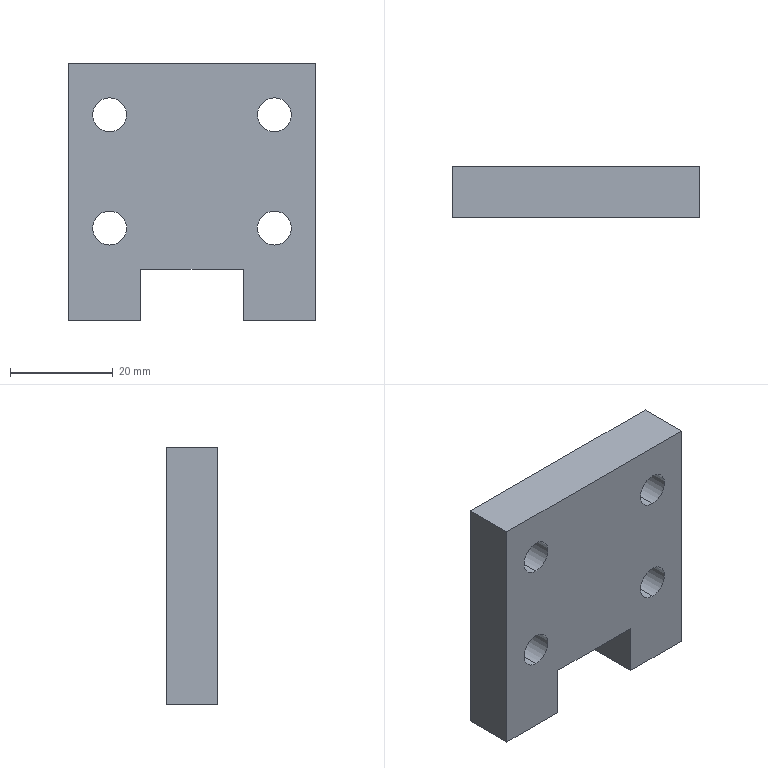Part | SolidWorks | features Extrusion 1, HoleWzd 1, ICE 1 | 1 solid | 38 faces | box 48 x 10 x 50 mm | volume 19683 mm3 | cylinder 16 | plane 14 | cone 8 | commonest cylinder face diameters 6.6 x8 11 x8
STEP:
#1=CARTESIAN_POINT('',(-16.,9.975,-12.5));
#2=VERTEX_POINT('',#1);
#3=CARTESIAN_POINT('',(-16.,9.975,-1.5));
#4=VERTEX_POINT('',#3);
#5=CARTESIAN_POINT('',(-16.,9.975,-7.));
#6=DIRECTION('',(0.,1.,0.));
#7=DIRECTION('',(0.,0.,1.));
#8=AXIS2_PLACEMENT_3D('',#5,#6,#7);
#9=CIRCLE('',#8,5.5);
#10=EDGE_CURVE('',#2,#4,#9,.T.);
#11=ORIENTED_EDGE('',*,*,#10,.F.);
#12=CARTESIAN_POINT('',(-16.,10.,-12.525));
#13=VERTEX_POINT('',#12);
#14=CARTESIAN_POINT('',(-16.,10.,-12.525));
#15=DIRECTION('',(0.,0.7071,-0.7071));
#16=VECTOR('',#15,1000.);
#17=LINE('',#14,#16);
#18=EDGE_CURVE('',#2,#13,#17,.T.);
#19=ORIENTED_EDGE('',*,*,#18,.T.);
#20=CARTESIAN_POINT('',(-16.,10.,-1.475));
#21=VERTEX_POINT('',#20);
#22=CARTESIAN_POINT('',(-16.,10.,-7.));
#23=DIRECTION('',(0.,1.,0.));
#24=DIRECTION('',(0.,0.,1.));
#25=AXIS2_PLACEMENT_3D('',#22,#23,#24);
#26=CIRCLE('',#25,5.525);
#27=EDGE_CURVE('',#13,#21,#26,.T.);
#28=ORIENTED_EDGE('',*,*,#27,.T.);
#29=CARTESIAN_POINT('',(-16.,10.,-1.475));
#30=DIRECTION('',(0.,0.7071,0.7071));
#31=VECTOR('',#30,1000.);
#32=LINE('',#29,#31);
#33=EDGE_CURVE('',#4,#21,#32,.T.);
#34=ORIENTED_EDGE('',*,*,#33,.F.);
#35=EDGE_LOOP('',(#11,#19,#28,#34));
#36=FACE_OUTER_BOUND('',#35,.T.);
#37=CARTESIAN_POINT('',(-16.,10.,-7.));
#38=DIRECTION('',(0.,1.,0.));
#39=DIRECTION('',(0.,0.,1.));
#40=AXIS2_PLACEMENT_3D('',#37,#38,#39);
#41=CONICAL_SURFACE('',#40,5.525,0.7854);
#42=ADVANCED_FACE('',(#36),#41,.F.);
#43=CARTESIAN_POINT('',(-16.,6.1,-12.5));
#44=VERTEX_POINT('',#43);
#45=CARTESIAN_POINT('',(-16.,6.1,-1.5));
#46=VERTEX_POINT('',#45);
#47=CARTESIAN_POINT('',(-16.,6.1,-7.));
#48=DIRECTION('',(0.,1.,0.));
#49=DIRECTION('',(0.,0.,1.));
#50=AXIS2_PLACEMENT_3D('',#47,#48,#49);
#51=CIRCLE('',#50,5.5);
#52=EDGE_CURVE('',#44,#46,#51,.T.);
#53=ORIENTED_EDGE('',*,*,#52,.F.);
#54=CARTESIAN_POINT('',(-16.,10.,-12.5));
#55=DIRECTION('',(0.,1.,0.));
#56=VECTOR('',#55,1000.);
#57=LINE('',#54,#56);
#58=EDGE_CURVE('',#44,#2,#57,.T.);
#59=ORIENTED_EDGE('',*,*,#58,.T.);
#60=ORIENTED_EDGE('',*,*,#10,.T.);
#61=CARTESIAN_POINT('',(-16.,10.,-1.5));
#62=DIRECTION('',(0.,1.,0.));
#63=VECTOR('',#62,1000.);
#64=LINE('',#61,#63);
#65=EDGE_CURVE('',#46,#4,#64,.T.);
#66=ORIENTED_EDGE('',*,*,#65,.F.);
#67=EDGE_LOOP('',(#53,#59,#60,#66));
#68=FACE_OUTER_BOUND('',#67,.T.);
#69=CARTESIAN_POINT('',(-16.,10.,-7.));
#70=DIRECTION('',(0.,1.,0.));
#71=DIRECTION('',(0.,0.,1.));
#72=AXIS2_PLACEMENT_3D('',#69,#70,#71);
#73=CYLINDRICAL_SURFACE('',#72,5.5);
#74=ADVANCED_FACE('',(#68),#73,.F.);
#75=CARTESIAN_POINT('',(-16.,0.,-10.3));
#76=VERTEX_POINT('',#75);
#77=CARTESIAN_POINT('',(-16.,0.,-3.7));
#78=VERTEX_POINT('',#77);
#79=CARTESIAN_POINT('',(-16.,0.,-7.));
#80=DIRECTION('',(0.,1.,0.));
#81=DIRECTION('',(0.,0.,1.));
#82=AXIS2_PLACEMENT_3D('',#79,#80,#81);
#83=CIRCLE('',#82,3.3);
#84=EDGE_CURVE('',#76,#78,#83,.T.);
#85=ORIENTED_EDGE('',*,*,#84,.F.);
#86=CARTESIAN_POINT('',(-16.,6.1,-10.3));
#87=VERTEX_POINT('',#86);
#88=CARTESIAN_POINT('',(-16.,10.,-10.3));
#89=DIRECTION('',(0.,1.,0.));
#90=VECTOR('',#89,1000.);
#91=LINE('',#88,#90);
#92=EDGE_CURVE('',#76,#87,#91,.T.);
#93=ORIENTED_EDGE('',*,*,#92,.T.);
#94=CARTESIAN_POINT('',(-16.,6.1,-3.7));
#95=VERTEX_POINT('',#94);
#96=CARTESIAN_POINT('',(-16.,6.1,-7.));
#97=DIRECTION('',(0.,1.,0.));
#98=DIRECTION('',(0.,0.,1.));
#99=AXIS2_PLACEMENT_3D('',#96,#97,#98);
#100=CIRCLE('',#99,3.3);
#101=EDGE_CURVE('',#87,#95,#100,.T.);
#102=ORIENTED_EDGE('',*,*,#101,.T.);
#103=CARTESIAN_POINT('',(-16.,10.,-3.7));
#104=DIRECTION('',(0.,1.,0.));
#105=VECTOR('',#104,1000.);
#106=LINE('',#103,#105);
#107=EDGE_CURVE('',#78,#95,#106,.T.);
#108=ORIENTED_EDGE('',*,*,#107,.F.);
#109=EDGE_LOOP('',(#85,#93,#102,#108));
#110=FACE_OUTER_BOUND('',#109,.T.);
#111=CARTESIAN_POINT('',(-16.,10.,-7.));
#112=DIRECTION('',(0.,1.,0.));
#113=DIRECTION('',(0.,0.,1.));
#114=AXIS2_PLACEMENT_3D('',#111,#112,#113);
#115=CYLINDRICAL_SURFACE('',#114,3.3);
#116=ADVANCED_FACE('',(#110),#115,.F.);
#117=CARTESIAN_POINT('',(-16.,9.975,9.5));
#118=VERTEX_POINT('',#117);
#119=CARTESIAN_POINT('',(-16.,9.975,20.5));
#120=VERTEX_POINT('',#119);
#121=CARTESIAN_POINT('',(-16.,9.975,15.));
#122=DIRECTION('',(0.,1.,0.));
#123=DIRECTION('',(0.,0.,1.));
#124=AXIS2_PLACEMENT_3D('',#121,#122,#123);
#125=CIRCLE('',#124,5.5);
#126=EDGE_CURVE('',#118,#120,#125,.T.);
#127=ORIENTED_EDGE('',*,*,#126,.F.);
#128=CARTESIAN_POINT('',(-16.,10.,9.475));
#129=VERTEX_POINT('',#128);
#130=CARTESIAN_POINT('',(-16.,10.,9.475));
#131=DIRECTION('',(0.,0.7071,-0.7071));
#132=VECTOR('',#131,1000.);
#133=LINE('',#130,#132);
#134=EDGE_CURVE('',#118,#129,#133,.T.);
#135=ORIENTED_EDGE('',*,*,#134,.T.);
#136=CARTESIAN_POINT('',(-16.,10.,20.525));
#137=VERTEX_POINT('',#136);
#138=CARTESIAN_POINT('',(-16.,10.,15.));
#139=DIRECTION('',(0.,1.,0.));
#140=DIRECTION('',(0.,0.,1.));
#141=AXIS2_PLACEMENT_3D('',#138,#139,#140);
#142=CIRCLE('',#141,5.525);
#143=EDGE_CURVE('',#129,#137,#142,.T.);
#144=ORIENTED_EDGE('',*,*,#143,.T.);
#145=CARTESIAN_POINT('',(-16.,10.,20.525));
#146=DIRECTION('',(0.,0.7071,0.7071));
#147=VECTOR('',#146,1000.);
#148=LINE('',#145,#147);
#149=EDGE_CURVE('',#120,#137,#148,.T.);
#150=ORIENTED_EDGE('',*,*,#149,.F.);
#151=EDGE_LOOP('',(#127,#135,#144,#150));
#152=FACE_OUTER_BOUND('',#151,.T.);
#153=CARTESIAN_POINT('',(-16.,10.,15.));
#154=DIRECTION('',(0.,1.,0.));
#155=DIRECTION('',(0.,0.,1.));
#156=AXIS2_PLACEMENT_3D('',#153,#154,#155);
#157=CONICAL_SURFACE('',#156,5.525,0.7854);
#158=ADVANCED_FACE('',(#152),#157,.F.);
#159=CARTESIAN_POINT('',(-16.,6.1,9.5));
#160=VERTEX_POINT('',#159);
#161=CARTESIAN_POINT('',(-16.,6.1,20.5));
#162=VERTEX_POINT('',#161);
#163=CARTESIAN_POINT('',(-16.,6.1,15.));
#164=DIRECTION('',(0.,1.,0.));
#165=DIRECTION('',(0.,0.,1.));
#166=AXIS2_PLACEMENT_3D('',#163,#164,#165);
#167=CIRCLE('',#166,5.5);
#168=EDGE_CURVE('',#160,#162,#167,.T.);
#169=ORIENTED_EDGE('',*,*,#168,.F.);
#170=CARTESIAN_POINT('',(-16.,10.,9.5));
#171=DIRECTION('',(0.,1.,0.));
#172=VECTOR('',#171,1000.);
#173=LINE('',#170,#172);
#174=EDGE_CURVE('',#160,#118,#173,.T.);
#175=ORIENTED_EDGE('',*,*,#174,.T.);
#176=ORIENTED_EDGE('',*,*,#126,.T.);
#177=CARTESIAN_POINT('',(-16.,10.,20.5));
#178=DIRECTION('',(0.,1.,0.));
#179=VECTOR('',#178,1000.);
#180=LINE('',#177,#179);
#181=EDGE_CURVE('',#162,#120,#180,.T.);
#182=ORIENTED_EDGE('',*,*,#181,.F.);
#183=EDGE_LOOP('',(#169,#175,#176,#182));
#184=FACE_OUTER_BOUND('',#183,.T.);
#185=CARTESIAN_POINT('',(-16.,10.,15.));
#186=DIRECTION('',(0.,1.,0.));
#187=DIRECTION('',(0.,0.,1.));
#188=AXIS2_PLACEMENT_3D('',#185,#186,#187);
#189=CYLINDRICAL_SURFACE('',#188,5.5);
#190=ADVANCED_FACE('',(#184),#189,.F.);
#191=CARTESIAN_POINT('',(-16.,0.,11.7));
#192=VERTEX_POINT('',#191);
#193=CARTESIAN_POINT('',(-16.,0.,18.3));
#194=VERTEX_POINT('',#193);
#195=CARTESIAN_POINT('',(-16.,0.,15.));
#196=DIRECTION('',(0.,1.,0.));
#197=DIRECTION('',(0.,0.,1.));
#198=AXIS2_PLACEMENT_3D('',#195,#196,#197);
#199=CIRCLE('',#198,3.3);
#200=EDGE_CURVE('',#192,#194,#199,.T.);
#201=ORIENTED_EDGE('',*,*,#200,.F.);
#202=CARTESIAN_POINT('',(-16.,6.1,11.7));
#203=VERTEX_POINT('',#202);
#204=CARTESIAN_POINT('',(-16.,10.,11.7));
#205=DIRECTION('',(0.,1.,0.));
#206=VECTOR('',#205,1000.);
#207=LINE('',#204,#206);
#208=EDGE_CURVE('',#192,#203,#207,.T.);
#209=ORIENTED_EDGE('',*,*,#208,.T.);
#210=CARTESIAN_POINT('',(-16.,6.1,18.3));
#211=VERTEX_POINT('',#210);
#212=CARTESIAN_POINT('',(-16.,6.1,15.));
#213=DIRECTION('',(0.,1.,0.));
#214=DIRECTION('',(0.,0.,1.));
#215=AXIS2_PLACEMENT_3D('',#212,#213,#214);
#216=CIRCLE('',#215,3.3);
#217=EDGE_CURVE('',#203,#211,#216,.T.);
#218=ORIENTED_EDGE('',*,*,#217,.T.);
#219=CARTESIAN_POINT('',(-16.,10.,18.3));
#220=DIRECTION('',(0.,1.,0.));
#221=VECTOR('',#220,1000.);
#222=LINE('',#219,#221);
#223=EDGE_CURVE('',#194,#211,#222,.T.);
#224=ORIENTED_EDGE('',*,*,#223,.F.);
#225=EDGE_LOOP('',(#201,#209,#218,#224));
#226=FACE_OUTER_BOUND('',#225,.T.);
#227=CARTESIAN_POINT('',(-16.,10.,15.));
#228=DIRECTION('',(0.,1.,0.));
#229=DIRECTION('',(0.,0.,1.));
#230=AXIS2_PLACEMENT_3D('',#227,#228,#229);
#231=CYLINDRICAL_SURFACE('',#230,3.3);
#232=ADVANCED_FACE('',(#226),#231,.F.);
#233=CARTESIAN_POINT('',(16.,9.975,9.5));
#234=VERTEX_POINT('',#233);
#235=CARTESIAN_POINT('',(16.,9.975,20.5));
#236=VERTEX_POINT('',#235);
#237=CARTESIAN_POINT('',(16.,9.975,15.));
#238=DIRECTION('',(0.,1.,0.));
#239=DIRECTION('',(0.,0.,1.));
#240=AXIS2_PLACEMENT_3D('',#237,#238,#239);
#241=CIRCLE('',#240,5.5);
#242=EDGE_CURVE('',#234,#236,#241,.T.);
#243=ORIENTED_EDGE('',*,*,#242,.F.);
#244=CARTESIAN_POINT('',(16.,10.,9.475));
#245=VERTEX_POINT('',#244);
#246=CARTESIAN_POINT('',(16.,10.,9.475));
#247=DIRECTION('',(0.,0.7071,-0.7071));
#248=VECTOR('',#247,1000.);
#249=LINE('',#246,#248);
#250=EDGE_CURVE('',#234,#245,#249,.T.);
#251=ORIENTED_EDGE('',*,*,#250,.T.);
#252=CARTESIAN_POINT('',(16.,10.,20.525));
#253=VERTEX_POINT('',#252);
#254=CARTESIAN_POINT('',(16.,10.,15.));
#255=DIRECTION('',(0.,1.,0.));
#256=DIRECTION('',(0.,0.,1.));
#257=AXIS2_PLACEMENT_3D('',#254,#255,#256);
#258=CIRCLE('',#257,5.525);
#259=EDGE_CURVE('',#245,#253,#258,.T.);
#260=ORIENTED_EDGE('',*,*,#259,.T.);
#261=CARTESIAN_POINT('',(16.,10.,20.525));
#262=DIRECTION('',(0.,0.7071,0.7071));
#263=VECTOR('',#262,1000.);
#264=LINE('',#261,#263);
#265=EDGE_CURVE('',#236,#253,#264,.T.);
#266=ORIENTED_EDGE('',*,*,#265,.F.);
#267=EDGE_LOOP('',(#243,#251,#260,#266));
#268=FACE_OUTER_BOUND('',#267,.T.);
#269=CARTESIAN_POINT('',(16.,10.,15.));
#270=DIRECTION('',(0.,1.,0.));
#271=DIRECTION('',(0.,0.,1.));
#272=AXIS2_PLACEMENT_3D('',#269,#270,#271);
#273=CONICAL_SURFACE('',#272,5.525,0.7854);
#274=ADVANCED_FACE('',(#268),#273,.F.);
#275=CARTESIAN_POINT('',(16.,6.1,9.5));
#276=VERTEX_POINT('',#275);
#277=CARTESIAN_POINT('',(16.,6.1,20.5));
#278=VERTEX_POINT('',#277);
#279=CARTESIAN_POINT('',(16.,6.1,15.));
#280=DIRECTION('',(0.,1.,0.));
#281=DIRECTION('',(0.,0.,1.));
#282=AXIS2_PLACEMENT_3D('',#279,#280,#281);
#283=CIRCLE('',#282,5.5);
#284=EDGE_CURVE('',#276,#278,#283,.T.);
#285=ORIENTED_EDGE('',*,*,#284,.F.);
#286=CARTESIAN_POINT('',(16.,10.,9.5));
#287=DIRECTION('',(0.,1.,0.));
#288=VECTOR('',#287,1000.);
#289=LINE('',#286,#288);
#290=EDGE_CURVE('',#276,#234,#289,.T.);
#291=ORIENTED_EDGE('',*,*,#290,.T.);
#292=ORIENTED_EDGE('',*,*,#242,.T.);
#293=CARTESIAN_POINT('',(16.,10.,20.5));
#294=DIRECTION('',(0.,1.,0.));
#295=VECTOR('',#294,1000.);
#296=LINE('',#293,#295);
#297=EDGE_CURVE('',#278,#236,#296,.T.);
#298=ORIENTED_EDGE('',*,*,#297,.F.);
#299=EDGE_LOOP('',(#285,#291,#292,#298));
#300=FACE_OUTER_BOUND('',#299,.T.);
#301=CARTESIAN_POINT('',(16.,10.,15.));
#302=DIRECTION('',(0.,1.,0.));
#303=DIRECTION('',(0.,0.,1.));
#304=AXIS2_PLACEMENT_3D('',#301,#302,#303);
#305=CYLINDRICAL_SURFACE('',#304,5.5);
#306=ADVANCED_FACE('',(#300),#305,.F.);
#307=CARTESIAN_POINT('',(16.,0.,11.7));
#308=VERTEX_POINT('',#307);
#309=CARTESIAN_POINT('',(16.,0.,18.3));
#310=VERTEX_POINT('',#309);
#311=CARTESIAN_POINT('',(16.,0.,15.));
#312=DIRECTION('',(0.,1.,0.));
#313=DIRECTION('',(0.,0.,1.));
#314=AXIS2_PLACEMENT_3D('',#311,#312,#313);
#315=CIRCLE('',#314,3.3);
#316=EDGE_CURVE('',#308,#310,#315,.T.);
#317=ORIENTED_EDGE('',*,*,#316,.F.);
#318=CARTESIAN_POINT('',(16.,6.1,11.7));
#319=VERTEX_POINT('',#318);
#320=CARTESIAN_POINT('',(16.,10.,11.7));
#321=DIRECTION('',(0.,1.,0.));
#322=VECTOR('',#321,1000.);
#323=LINE('',#320,#322);
#324=EDGE_CURVE('',#308,#319,#323,.T.);
#325=ORIENTED_EDGE('',*,*,#324,.T.);
#326=CARTESIAN_POINT('',(16.,6.1,18.3));
#327=VERTEX_POINT('',#326);
#328=CARTESIAN_POINT('',(16.,6.1,15.));
#329=DIRECTION('',(0.,1.,0.));
#330=DIRECTION('',(0.,0.,1.));
#331=AXIS2_PLACEMENT_3D('',#328,#329,#330);
#332=CIRCLE('',#331,3.3);
#333=EDGE_CURVE('',#319,#327,#332,.T.);
#334=ORIENTED_EDGE('',*,*,#333,.T.);
#335=CARTESIAN_POINT('',(16.,10.,18.3));
#336=DIRECTION('',(0.,1.,0.));
#337=VECTOR('',#336,1000.);
#338=LINE('',#335,#337);
#339=EDGE_CURVE('',#310,#327,#338,.T.);
#340=ORIENTED_EDGE('',*,*,#339,.F.);
#341=EDGE_LOOP('',(#317,#325,#334,#340));
#342=FACE_OUTER_BOUND('',#341,.T.);
#343=CARTESIAN_POINT('',(16.,10.,15.));
#344=DIRECTION('',(0.,1.,0.));
#345=DIRECTION('',(0.,0.,1.));
#346=AXIS2_PLACEMENT_3D('',#343,#344,#345);
#347=CYLINDRICAL_SURFACE('',#346,3.3);
#348=ADVANCED_FACE('',(#342),#347,.F.);
#349=CARTESIAN_POINT('',(16.,9.975,-12.5));
#350=VERTEX_POINT('',#349);
#351=CARTESIAN_POINT('',(16.,9.975,-1.5));
#352=VERTEX_POINT('',#351);
#353=CARTESIAN_POINT('',(16.,9.975,-7.));
#354=DIRECTION('',(0.,1.,0.));
#355=DIRECTION('',(0.,0.,1.));
#356=AXIS2_PLACEMENT_3D('',#353,#354,#355);
#357=CIRCLE('',#356,5.5);
#358=EDGE_CURVE('',#350,#352,#357,.T.);
#359=ORIENTED_EDGE('',*,*,#358,.F.);
#360=CARTESIAN_POINT('',(16.,10.,-12.525));
#361=VERTEX_POINT('',#360);
#362=CARTESIAN_POINT('',(16.,10.,-12.525));
#363=DIRECTION('',(0.,0.7071,-0.7071));
#364=VECTOR('',#363,1000.);
#365=LINE('',#362,#364);
#366=EDGE_CURVE('',#350,#361,#365,.T.);
#367=ORIENTED_EDGE('',*,*,#366,.T.);
#368=CARTESIAN_POINT('',(16.,10.,-1.475));
#369=VERTEX_POINT('',#368);
#370=CARTESIAN_POINT('',(16.,10.,-7.));
#371=DIRECTION('',(0.,1.,0.));
#372=DIRECTION('',(0.,0.,1.));
#373=AXIS2_PLACEMENT_3D('',#370,#371,#372);
#374=CIRCLE('',#373,5.525);
#375=EDGE_CURVE('',#361,#369,#374,.T.);
#376=ORIENTED_EDGE('',*,*,#375,.T.);
#377=CARTESIAN_POINT('',(16.,10.,-1.475));
#378=DIRECTION('',(0.,0.7071,0.7071));
#379=VECTOR('',#378,1000.);
#380=LINE('',#377,#379);
#381=EDGE_CURVE('',#352,#369,#380,.T.);
#382=ORIENTED_EDGE('',*,*,#381,.F.);
#383=EDGE_LOOP('',(#359,#367,#376,#382));
#384=FACE_OUTER_BOUND('',#383,.T.);
#385=CARTESIAN_POINT('',(16.,10.,-7.));
#386=DIRECTION('',(0.,1.,0.));
#387=DIRECTION('',(0.,0.,1.));
#388=AXIS2_PLACEMENT_3D('',#385,#386,#387);
#389=CONICAL_SURFACE('',#388,5.525,0.7854);
#390=ADVANCED_FACE('',(#384),#389,.F.);
#391=CARTESIAN_POINT('',(16.,6.1,-12.5));
#392=VERTEX_POINT('',#391);
#393=CARTESIAN_POINT('',(16.,6.1,-1.5));
#394=VERTEX_POINT('',#393);
#395=CARTESIAN_POINT('',(16.,6.1,-7.));
#396=DIRECTION('',(0.,1.,0.));
#397=DIRECTION('',(0.,0.,1.));
#398=AXIS2_PLACEMENT_3D('',#395,#396,#397);
#399=CIRCLE('',#398,5.5);
#400=EDGE_CURVE('',#392,#394,#399,.T.);
#401=ORIENTED_EDGE('',*,*,#400,.F.);
#402=CARTESIAN_POINT('',(16.,10.,-12.5));
#403=DIRECTION('',(0.,1.,0.));
#404=VECTOR('',#403,1000.);
#405=LINE('',#402,#404);
#406=EDGE_CURVE('',#392,#350,#405,.T.);
#407=ORIENTED_EDGE('',*,*,#406,.T.);
#408=ORIENTED_EDGE('',*,*,#358,.T.);
#409=CARTESIAN_POINT('',(16.,10.,-1.5));
#410=DIRECTION('',(0.,1.,0.));
#411=VECTOR('',#410,1000.);
#412=LINE('',#409,#411);
#413=EDGE_CURVE('',#394,#352,#412,.T.);
#414=ORIENTED_EDGE('',*,*,#413,.F.);
#415=EDGE_LOOP('',(#401,#407,#408,#414));
#416=FACE_OUTER_BOUND('',#415,.T.);
#417=CARTESIAN_POINT('',(16.,10.,-7.));
#418=DIRECTION('',(0.,1.,0.));
#419=DIRECTION('',(0.,0.,1.));
#420=AXIS2_PLACEMENT_3D('',#417,#418,#419);
#421=CYLINDRICAL_SURFACE('',#420,5.5);
#422=ADVANCED_FACE('',(#416),#421,.F.);
#423=CARTESIAN_POINT('',(16.,0.,-10.3));
#424=VERTEX_POINT('',#423);
#425=CARTESIAN_POINT('',(16.,0.,-3.7));
#426=VERTEX_POINT('',#425);
#427=CARTESIAN_POINT('',(16.,0.,-7.));
#428=DIRECTION('',(0.,1.,0.));
#429=DIRECTION('',(0.,0.,1.));
#430=AXIS2_PLACEMENT_3D('',#427,#428,#429);
#431=CIRCLE('',#430,3.3);
#432=EDGE_CURVE('',#424,#426,#431,.T.);
#433=ORIENTED_EDGE('',*,*,#432,.F.);
#434=CARTESIAN_POINT('',(16.,6.1,-10.3));
#435=VERTEX_POINT('',#434);
#436=CARTESIAN_POINT('',(16.,10.,-10.3));
#437=DIRECTION('',(0.,1.,0.));
#438=VECTOR('',#437,1000.);
#439=LINE('',#436,#438);
#440=EDGE_CURVE('',#424,#435,#439,.T.);
#441=ORIENTED_EDGE('',*,*,#440,.T.);
#442=CARTESIAN_POINT('',(16.,6.1,-3.7));
#443=VERTEX_POINT('',#442);
#444=CARTESIAN_POINT('',(16.,6.1,-7.));
#445=DIRECTION('',(0.,1.,0.));
#446=DIRECTION('',(0.,0.,1.));
#447=AXIS2_PLACEMENT_3D('',#444,#445,#446);
#448=CIRCLE('',#447,3.3);
#449=EDGE_CURVE('',#435,#443,#448,.T.);
#450=ORIENTED_EDGE('',*,*,#449,.T.);
#451=CARTESIAN_POINT('',(16.,10.,-3.7));
#452=DIRECTION('',(0.,1.,0.));
#453=VECTOR('',#452,1000.);
#454=LINE('',#451,#453);
#455=EDGE_CURVE('',#426,#443,#454,.T.);
#456=ORIENTED_EDGE('',*,*,#455,.F.);
#457=EDGE_LOOP('',(#433,#441,#450,#456));
#458=FACE_OUTER_BOUND('',#457,.T.);
#459=CARTESIAN_POINT('',(16.,10.,-7.));
#460=DIRECTION('',(0.,1.,0.));
#461=DIRECTION('',(0.,0.,1.));
#462=AXIS2_PLACEMENT_3D('',#459,#460,#461);
#463=CYLINDRICAL_SURFACE('',#462,3.3);
#464=ADVANCED_FACE('',(#458),#463,.F.);
#465=CARTESIAN_POINT('',(24.,0.,-25.));
#466=VERTEX_POINT('',#465);
#467=CARTESIAN_POINT('',(10.,0.,-25.));
#468=VERTEX_POINT('',#467);
#469=CARTESIAN_POINT('',(-24.,0.,-25.));
#470=DIRECTION('',(-1.,0.,0.));
#471=VECTOR('',#470,1000.);
#472=LINE('',#469,#471);
#473=EDGE_CURVE('',#466,#468,#472,.T.);
#474=ORIENTED_EDGE('',*,*,#473,.T.);
#475=CARTESIAN_POINT('',(10.,10.,-25.));
#476=VERTEX_POINT('',#475);
#477=CARTESIAN_POINT('',(10.,10.,-25.));
#478=DIRECTION('',(0.,1.,0.));
#479=VECTOR('',#478,1000.);
#480=LINE('',#477,#479);
#481=EDGE_CURVE('',#468,#476,#480,.T.);
#482=ORIENTED_EDGE('',*,*,#481,.T.);
#483=CARTESIAN_POINT('',(24.,10.,-25.));
#484=VERTEX_POINT('',#483);
#485=CARTESIAN_POINT('',(-24.,10.,-25.));
#486=DIRECTION('',(-1.,0.,0.));
#487=VECTOR('',#486,1000.);
#488=LINE('',#485,#487);
#489=EDGE_CURVE('',#484,#476,#488,.T.);
#490=ORIENTED_EDGE('',*,*,#489,.F.);
#491=CARTESIAN_POINT('',(24.,10.,-25.));
#492=DIRECTION('',(0.,-1.,0.));
#493=VECTOR('',#492,1000.);
#494=LINE('',#491,#493);
#495=EDGE_CURVE('',#484,#466,#494,.T.);
#496=ORIENTED_EDGE('',*,*,#495,.T.);
#497=EDGE_LOOP('',(#474,#482,#490,#496));
#498=FACE_OUTER_BOUND('',#497,.T.);
#499=CARTESIAN_POINT('',(-24.,10.,-25.));
#500=DIRECTION('',(0.,0.,1.));
#501=DIRECTION('',(1.,0.,0.));
#502=AXIS2_PLACEMENT_3D('',#499,#500,#501);
#503=PLANE('',#502);
#504=ADVANCED_FACE('',(#498),#503,.F.);
#505=CARTESIAN_POINT('',(24.,0.,25.));
#506=VERTEX_POINT('',#505);
#507=CARTESIAN_POINT('',(24.,0.,-25.));
#508=DIRECTION('',(0.,0.,-1.));
#509=VECTOR('',#508,1000.);
#510=LINE('',#507,#509);
#511=EDGE_CURVE('',#506,#466,#510,.T.);
#512=ORIENTED_EDGE('',*,*,#511,.T.);
#513=ORIENTED_EDGE('',*,*,#495,.F.);
#514=CARTESIAN_POINT('',(24.,10.,25.));
#515=VERTEX_POINT('',#514);
#516=CARTESIAN_POINT('',(24.,10.,-25.));
#517=DIRECTION('',(0.,0.,-1.));
#518=VECTOR('',#517,1000.);
#519=LINE('',#516,#518);
#520=EDGE_CURVE('',#515,#484,#519,.T.);
#521=ORIENTED_EDGE('',*,*,#520,.F.);
#522=CARTESIAN_POINT('',(24.,10.,25.));
#523=DIRECTION('',(0.,-1.,0.));
#524=VECTOR('',#523,1000.);
#525=LINE('',#522,#524);
#526=EDGE_CURVE('',#515,#506,#525,.T.);
#527=ORIENTED_EDGE('',*,*,#526,.T.);
#528=EDGE_LOOP('',(#512,#513,#521,#527));
#529=FACE_OUTER_BOUND('',#528,.T.);
#530=CARTESIAN_POINT('',(24.,10.,-25.));
#531=DIRECTION('',(-1.,0.,0.));
#532=DIRECTION('',(0.,0.,1.));
#533=AXIS2_PLACEMENT_3D('',#530,#531,#532);
#534=PLANE('',#533);
#535=ADVANCED_FACE('',(#529),#534,.F.);
#536=CARTESIAN_POINT('',(-10.,10.,-25.));
#537=VERTEX_POINT('',#536);
#538=CARTESIAN_POINT('',(-24.,10.,-25.));
#539=VERTEX_POINT('',#538);
#540=CARTESIAN_POINT('',(-24.,10.,-25.));
#541=DIRECTION('',(-1.,0.,0.));
#542=VECTOR('',#541,1000.);
#543=LINE('',#540,#542);
#544=EDGE_CURVE('',#537,#539,#543,.T.);
#545=ORIENTED_EDGE('',*,*,#544,.F.);
#546=CARTESIAN_POINT('',(-10.,0.,-25.));
#547=VERTEX_POINT('',#546);
#548=CARTESIAN_POINT('',(-10.,10.,-25.));
#549=DIRECTION('',(0.,-1.,0.));
#550=VECTOR('',#549,1000.);
#551=LINE('',#548,#550);
#552=EDGE_CURVE('',#537,#547,#551,.T.);
#553=ORIENTED_EDGE('',*,*,#552,.T.);
#554=CARTESIAN_POINT('',(-24.,0.,-25.));
#555=VERTEX_POINT('',#554);
#556=CARTESIAN_POINT('',(-24.,0.,-25.));
#557=DIRECTION('',(-1.,0.,0.));
#558=VECTOR('',#557,1000.);
#559=LINE('',#556,#558);
#560=EDGE_CURVE('',#547,#555,#559,.T.);
#561=ORIENTED_EDGE('',*,*,#560,.T.);
#562=CARTESIAN_POINT('',(-24.,10.,-25.));
#563=DIRECTION('',(0.,-1.,0.));
#564=VECTOR('',#563,1000.);
#565=LINE('',#562,#564);
#566=EDGE_CURVE('',#539,#555,#565,.T.);
#567=ORIENTED_EDGE('',*,*,#566,.F.);
#568=EDGE_LOOP('',(#545,#553,#561,#567));
#569=FACE_OUTER_BOUND('',#568,.T.);
#570=CARTESIAN_POINT('',(-24.,10.,-25.));
#571=DIRECTION('',(0.,0.,1.));
#572=DIRECTION('',(1.,0.,0.));
#573=AXIS2_PLACEMENT_3D('',#570,#571,#572);
#574=PLANE('',#573);
#575=ADVANCED_FACE('',(#569),#574,.F.);
#576=CARTESIAN_POINT('',(-24.,0.,25.));
#577=VERTEX_POINT('',#576);
#578=CARTESIAN_POINT('',(-24.,0.,-25.));
#579=DIRECTION('',(0.,0.,1.));
#580=VECTOR('',#579,1000.);
#581=LINE('',#578,#580);
#582=EDGE_CURVE('',#555,#577,#581,.T.);
#583=ORIENTED_EDGE('',*,*,#582,.T.);
#584=CARTESIAN_POINT('',(-24.,10.,25.));
#585=VERTEX_POINT('',#584);
#586=CARTESIAN_POINT('',(-24.,10.,25.));
#587=DIRECTION('',(0.,-1.,0.));
#588=VECTOR('',#587,1000.);
#589=LINE('',#586,#588);
#590=EDGE_CURVE('',#585,#577,#589,.T.);
#591=ORIENTED_EDGE('',*,*,#590,.F.);
#592=CARTESIAN_POINT('',(-24.,10.,-25.));
#593=DIRECTION('',(0.,0.,1.));
#594=VECTOR('',#593,1000.);
#595=LINE('',#592,#594);
#596=EDGE_CURVE('',#539,#585,#595,.T.);
#597=ORIENTED_EDGE('',*,*,#596,.F.);
#598=ORIENTED_EDGE('',*,*,#566,.T.);
#599=EDGE_LOOP('',(#583,#591,#597,#598));
#600=FACE_OUTER_BOUND('',#599,.T.);
#601=CARTESIAN_POINT('',(-24.,10.,-25.));
#602=DIRECTION('',(1.,0.,0.));
#603=DIRECTION('',(0.,0.,-1.));
#604=AXIS2_PLACEMENT_3D('',#601,#602,#603);
#605=PLANE('',#604);
#606=ADVANCED_FACE('',(#600),#605,.F.);
#607=CARTESIAN_POINT('',(-24.,0.,25.));
#608=DIRECTION('',(1.,0.,0.));
#609=VECTOR('',#608,1000.);
#610=LINE('',#607,#609);
#611=EDGE_CURVE('',#577,#506,#610,.T.);
#612=ORIENTED_EDGE('',*,*,#611,.T.);
#613=ORIENTED_EDGE('',*,*,#526,.F.);
#614=CARTESIAN_POINT('',(-24.,10.,25.));
#615=DIRECTION('',(1.,0.,0.));
#616=VECTOR('',#615,1000.);
#617=LINE('',#614,#616);
#618=EDGE_CURVE('',#585,#515,#617,.T.);
#619=ORIENTED_EDGE('',*,*,#618,.F.);
#620=ORIENTED_EDGE('',*,*,#590,.T.);
#621=EDGE_LOOP('',(#612,#613,#619,#620));
#622=FACE_OUTER_BOUND('',#621,.T.);
#623=CARTESIAN_POINT('',(-24.,10.,25.));
#624=DIRECTION('',(0.,0.,-1.));
#625=DIRECTION('',(-1.,0.,0.));
#626=AXIS2_PLACEMENT_3D('',#623,#624,#625);
#627=PLANE('',#626);
#628=ADVANCED_FACE('',(#622),#627,.F.);
#629=CARTESIAN_POINT('',(-16.,10.,-7.));
#630=DIRECTION('',(0.,1.,0.));
#631=DIRECTION('',(0.,0.,1.));
#632=AXIS2_PLACEMENT_3D('',#629,#630,#631);
#633=CIRCLE('',#632,5.525);
#634=EDGE_CURVE('',#21,#13,#633,.T.);
#635=ORIENTED_EDGE('',*,*,#634,.F.);
#636=ORIENTED_EDGE('',*,*,#27,.F.);
#637=EDGE_LOOP('',(#635,#636));
#638=FACE_BOUND('',#637,.T.);
#639=CARTESIAN_POINT('',(-16.,10.,15.));
#640=DIRECTION('',(0.,1.,0.));
#641=DIRECTION('',(0.,0.,1.));
#642=AXIS2_PLACEMENT_3D('',#639,#640,#641);
#643=CIRCLE('',#642,5.525);
#644=EDGE_CURVE('',#137,#129,#643,.T.);
#645=ORIENTED_EDGE('',*,*,#644,.F.);
#646=ORIENTED_EDGE('',*,*,#143,.F.);
#647=EDGE_LOOP('',(#645,#646));
#648=FACE_BOUND('',#647,.T.);
#649=CARTESIAN_POINT('',(16.,10.,15.));
#650=DIRECTION('',(0.,1.,0.));
#651=DIRECTION('',(0.,0.,1.));
#652=AXIS2_PLACEMENT_3D('',#649,#650,#651);
#653=CIRCLE('',#652,5.525);
#654=EDGE_CURVE('',#253,#245,#653,.T.);
#655=ORIENTED_EDGE('',*,*,#654,.F.);
#656=ORIENTED_EDGE('',*,*,#259,.F.);
#657=EDGE_LOOP('',(#655,#656));
#658=FACE_BOUND('',#657,.T.);
#659=CARTESIAN_POINT('',(16.,10.,-7.));
#660=DIRECTION('',(0.,1.,0.));
#661=DIRECTION('',(0.,0.,1.));
#662=AXIS2_PLACEMENT_3D('',#659,#660,#661);
#663=CIRCLE('',#662,5.525);
#664=EDGE_CURVE('',#369,#361,#663,.T.);
#665=ORIENTED_EDGE('',*,*,#664,.F.);
#666=ORIENTED_EDGE('',*,*,#375,.F.);
#667=EDGE_LOOP('',(#665,#666));
#668=FACE_BOUND('',#667,.T.);
#669=CARTESIAN_POINT('',(10.,10.,-15.));
#670=VERTEX_POINT('',#669);
#671=CARTESIAN_POINT('',(10.,10.,-35.));
#672=DIRECTION('',(0.,0.,-1.));
#673=VECTOR('',#672,1000.);
#674=LINE('',#671,#673);
#675=EDGE_CURVE('',#670,#476,#674,.T.);
#676=ORIENTED_EDGE('',*,*,#675,.F.);
#677=CARTESIAN_POINT('',(-10.,10.,-15.));
#678=VERTEX_POINT('',#677);
#679=CARTESIAN_POINT('',(-10.,10.,-15.));
#680=DIRECTION('',(1.,0.,0.));
#681=VECTOR('',#680,1000.);
#682=LINE('',#679,#681);
#683=EDGE_CURVE('',#678,#670,#682,.T.);
#684=ORIENTED_EDGE('',*,*,#683,.F.);
#685=CARTESIAN_POINT('',(-10.,10.,-35.));
#686=DIRECTION('',(0.,0.,1.));
#687=VECTOR('',#686,1000.);
#688=LINE('',#685,#687);
#689=EDGE_CURVE('',#537,#678,#688,.T.);
#690=ORIENTED_EDGE('',*,*,#689,.F.);
#691=ORIENTED_EDGE('',*,*,#544,.T.);
#692=ORIENTED_EDGE('',*,*,#596,.T.);
#693=ORIENTED_EDGE('',*,*,#618,.T.);
#694=ORIENTED_EDGE('',*,*,#520,.T.);
#695=ORIENTED_EDGE('',*,*,#489,.T.);
#696=EDGE_LOOP('',(#676,#684,#690,#691,#692,#693,#694,#695));
#697=FACE_OUTER_BOUND('',#696,.T.);
#698=CARTESIAN_POINT('',(0.,10.,0.));
#699=DIRECTION('',(0.,1.,0.));
#700=DIRECTION('',(0.,0.,1.));
#701=AXIS2_PLACEMENT_3D('',#698,#699,#700);
#702=PLANE('',#701);
#703=ADVANCED_FACE('',(#638,#648,#658,#668,#697),#702,.T.);
#704=CARTESIAN_POINT('',(-16.,0.,-7.));
#705=DIRECTION('',(0.,1.,0.));
#706=DIRECTION('',(0.,0.,1.));
#707=AXIS2_PLACEMENT_3D('',#704,#705,#706);
#708=CIRCLE('',#707,3.3);
#709=EDGE_CURVE('',#78,#76,#708,.T.);
#710=ORIENTED_EDGE('',*,*,#709,.T.);
#711=ORIENTED_EDGE('',*,*,#84,.T.);
#712=EDGE_LOOP('',(#710,#711));
#713=FACE_BOUND('',#712,.T.);
#714=CARTESIAN_POINT('',(-16.,0.,15.));
#715=DIRECTION('',(0.,1.,0.));
#716=DIRECTION('',(0.,0.,1.));
#717=AXIS2_PLACEMENT_3D('',#714,#715,#716);
#718=CIRCLE('',#717,3.3);
#719=EDGE_CURVE('',#194,#192,#718,.T.);
#720=ORIENTED_EDGE('',*,*,#719,.T.);
#721=ORIENTED_EDGE('',*,*,#200,.T.);
#722=EDGE_LOOP('',(#720,#721));
#723=FACE_BOUND('',#722,.T.);
#724=CARTESIAN_POINT('',(16.,0.,15.));
#725=DIRECTION('',(0.,1.,0.));
#726=DIRECTION('',(0.,0.,1.));
#727=AXIS2_PLACEMENT_3D('',#724,#725,#726);
#728=CIRCLE('',#727,3.3);
#729=EDGE_CURVE('',#310,#308,#728,.T.);
#730=ORIENTED_EDGE('',*,*,#729,.T.);
#731=ORIENTED_EDGE('',*,*,#316,.T.);
#732=EDGE_LOOP('',(#730,#731));
#733=FACE_BOUND('',#732,.T.);
#734=CARTESIAN_POINT('',(16.,0.,-7.));
#735=DIRECTION('',(0.,1.,0.));
#736=DIRECTION('',(0.,0.,1.));
#737=AXIS2_PLACEMENT_3D('',#734,#735,#736);
#738=CIRCLE('',#737,3.3);
#739=EDGE_CURVE('',#426,#424,#738,.T.);
#740=ORIENTED_EDGE('',*,*,#739,.T.);
#741=ORIENTED_EDGE('',*,*,#432,.T.);
#742=EDGE_LOOP('',(#740,#741));
#743=FACE_BOUND('',#742,.T.);
#744=CARTESIAN_POINT('',(-10.,0.,-15.));
#745=VERTEX_POINT('',#744);
#746=CARTESIAN_POINT('',(10.,0.,-15.));
#747=VERTEX_POINT('',#746);
#748=CARTESIAN_POINT('',(-10.,0.,-15.));
#749=DIRECTION('',(1.,0.,0.));
#750=VECTOR('',#749,1000.);
#751=LINE('',#748,#750);
#752=EDGE_CURVE('',#745,#747,#751,.T.);
#753=ORIENTED_EDGE('',*,*,#752,.T.);
#754=CARTESIAN_POINT('',(10.,0.,-35.));
#755=DIRECTION('',(0.,0.,-1.));
#756=VECTOR('',#755,1000.);
#757=LINE('',#754,#756);
#758=EDGE_CURVE('',#747,#468,#757,.T.);
#759=ORIENTED_EDGE('',*,*,#758,.T.);
#760=ORIENTED_EDGE('',*,*,#473,.F.);
#761=ORIENTED_EDGE('',*,*,#511,.F.);
#762=ORIENTED_EDGE('',*,*,#611,.F.);
#763=ORIENTED_EDGE('',*,*,#582,.F.);
#764=ORIENTED_EDGE('',*,*,#560,.F.);
#765=CARTESIAN_POINT('',(-10.,0.,0.));
#766=DIRECTION('',(0.,0.,1.));
#767=VECTOR('',#766,1000.);
#768=LINE('',#765,#767);
#769=EDGE_CURVE('',#547,#745,#768,.T.);
#770=ORIENTED_EDGE('',*,*,#769,.T.);
#771=EDGE_LOOP('',(#753,#759,#760,#761,#762,#763,#764,#770));
#772=FACE_OUTER_BOUND('',#771,.T.);
#773=CARTESIAN_POINT('',(0.,0.,0.));
#774=DIRECTION('',(0.,1.,0.));
#775=DIRECTION('',(0.,0.,1.));
#776=AXIS2_PLACEMENT_3D('',#773,#774,#775);
#777=PLANE('',#776);
#778=ADVANCED_FACE('',(#713,#723,#733,#743,#772),#777,.F.);
#779=ORIENTED_EDGE('',*,*,#758,.F.);
#780=CARTESIAN_POINT('',(10.,0.,-15.));
#781=DIRECTION('',(0.,1.,0.));
#782=VECTOR('',#781,1000.);
#783=LINE('',#780,#782);
#784=EDGE_CURVE('',#747,#670,#783,.T.);
#785=ORIENTED_EDGE('',*,*,#784,.T.);
#786=ORIENTED_EDGE('',*,*,#675,.T.);
#787=ORIENTED_EDGE('',*,*,#481,.F.);
#788=EDGE_LOOP('',(#779,#785,#786,#787));
#789=FACE_OUTER_BOUND('',#788,.T.);
#790=CARTESIAN_POINT('',(10.,0.,-35.));
#791=DIRECTION('',(1.,0.,0.));
#792=DIRECTION('',(0.,0.,-1.));
#793=AXIS2_PLACEMENT_3D('',#790,#791,#792);
#794=PLANE('',#793);
#795=ADVANCED_FACE('',(#789),#794,.F.);
#796=ORIENTED_EDGE('',*,*,#689,.T.);
#797=CARTESIAN_POINT('',(-10.,0.,-15.));
#798=DIRECTION('',(0.,1.,0.));
#799=VECTOR('',#798,1000.);
#800=LINE('',#797,#799);
#801=EDGE_CURVE('',#745,#678,#800,.T.);
#802=ORIENTED_EDGE('',*,*,#801,.F.);
#803=ORIENTED_EDGE('',*,*,#769,.F.);
#804=ORIENTED_EDGE('',*,*,#552,.F.);
#805=EDGE_LOOP('',(#796,#802,#803,#804));
#806=FACE_OUTER_BOUND('',#805,.T.);
#807=CARTESIAN_POINT('',(-10.,0.,-35.));
#808=DIRECTION('',(-1.,0.,0.));
#809=DIRECTION('',(0.,0.,1.));
#810=AXIS2_PLACEMENT_3D('',#807,#808,#809);
#811=PLANE('',#810);
#812=ADVANCED_FACE('',(#806),#811,.F.);
#813=ORIENTED_EDGE('',*,*,#683,.T.);
#814=ORIENTED_EDGE('',*,*,#784,.F.);
#815=ORIENTED_EDGE('',*,*,#752,.F.);
#816=ORIENTED_EDGE('',*,*,#801,.T.);
#817=EDGE_LOOP('',(#813,#814,#815,#816));
#818=FACE_OUTER_BOUND('',#817,.T.);
#819=CARTESIAN_POINT('',(-10.,0.,-15.));
#820=DIRECTION('',(0.,0.,1.));
#821=DIRECTION('',(1.,0.,0.));
#822=AXIS2_PLACEMENT_3D('',#819,#820,#821);
#823=PLANE('',#822);
#824=ADVANCED_FACE('',(#818),#823,.F.);
#825=ORIENTED_EDGE('',*,*,#440,.F.);
#826=ORIENTED_EDGE('',*,*,#739,.F.);
#827=ORIENTED_EDGE('',*,*,#455,.T.);
#828=CARTESIAN_POINT('',(16.,6.1,-7.));
#829=DIRECTION('',(0.,1.,0.));
#830=DIRECTION('',(0.,0.,1.));
#831=AXIS2_PLACEMENT_3D('',#828,#829,#830);
#832=CIRCLE('',#831,3.3);
#833=EDGE_CURVE('',#443,#435,#832,.T.);
#834=ORIENTED_EDGE('',*,*,#833,.T.);
#835=EDGE_LOOP('',(#825,#826,#827,#834));
#836=FACE_OUTER_BOUND('',#835,.T.);
#837=CARTESIAN_POINT('',(16.,10.,-7.));
#838=DIRECTION('',(0.,1.,0.));
#839=DIRECTION('',(0.,0.,1.));
#840=AXIS2_PLACEMENT_3D('',#837,#838,#839);
#841=CYLINDRICAL_SURFACE('',#840,3.3);
#842=ADVANCED_FACE('',(#836),#841,.F.);
#843=ORIENTED_EDGE('',*,*,#833,.F.);
#844=ORIENTED_EDGE('',*,*,#449,.F.);
#845=EDGE_LOOP('',(#843,#844));
#846=FACE_BOUND('',#845,.T.);
#847=CARTESIAN_POINT('',(16.,6.1,-7.));
#848=DIRECTION('',(0.,1.,0.));
#849=DIRECTION('',(0.,0.,1.));
#850=AXIS2_PLACEMENT_3D('',#847,#848,#849);
#851=CIRCLE('',#850,5.5);
#852=EDGE_CURVE('',#394,#392,#851,.T.);
#853=ORIENTED_EDGE('',*,*,#852,.T.);
#854=ORIENTED_EDGE('',*,*,#400,.T.);
#855=EDGE_LOOP('',(#853,#854));
#856=FACE_OUTER_BOUND('',#855,.T.);
#857=CARTESIAN_POINT('',(19.3,6.1,-7.));
#858=DIRECTION('',(0.,-1.,0.));
#859=DIRECTION('',(0.,0.,-1.));
#860=AXIS2_PLACEMENT_3D('',#857,#858,#859);
#861=PLANE('',#860);
#862=ADVANCED_FACE('',(#846,#856),#861,.F.);
#863=ORIENTED_EDGE('',*,*,#406,.F.);
#864=ORIENTED_EDGE('',*,*,#852,.F.);
#865=ORIENTED_EDGE('',*,*,#413,.T.);
#866=CARTESIAN_POINT('',(16.,9.975,-7.));
#867=DIRECTION('',(0.,1.,0.));
#868=DIRECTION('',(0.,0.,1.));
#869=AXIS2_PLACEMENT_3D('',#866,#867,#868);
#870=CIRCLE('',#869,5.5);
#871=EDGE_CURVE('',#352,#350,#870,.T.);
#872=ORIENTED_EDGE('',*,*,#871,.T.);
#873=EDGE_LOOP('',(#863,#864,#865,#872));
#874=FACE_OUTER_BOUND('',#873,.T.);
#875=CARTESIAN_POINT('',(16.,10.,-7.));
#876=DIRECTION('',(0.,1.,0.));
#877=DIRECTION('',(0.,0.,1.));
#878=AXIS2_PLACEMENT_3D('',#875,#876,#877);
#879=CYLINDRICAL_SURFACE('',#878,5.5);
#880=ADVANCED_FACE('',(#874),#879,.F.);
#881=ORIENTED_EDGE('',*,*,#366,.F.);
#882=ORIENTED_EDGE('',*,*,#871,.F.);
#883=ORIENTED_EDGE('',*,*,#381,.T.);
#884=ORIENTED_EDGE('',*,*,#664,.T.);
#885=EDGE_LOOP('',(#881,#882,#883,#884));
#886=FACE_OUTER_BOUND('',#885,.T.);
#887=CARTESIAN_POINT('',(16.,10.,-7.));
#888=DIRECTION('',(0.,1.,0.));
#889=DIRECTION('',(0.,0.,1.));
#890=AXIS2_PLACEMENT_3D('',#887,#888,#889);
#891=CONICAL_SURFACE('',#890,5.525,0.7854);
#892=ADVANCED_FACE('',(#886),#891,.F.);
#893=ORIENTED_EDGE('',*,*,#324,.F.);
#894=ORIENTED_EDGE('',*,*,#729,.F.);
#895=ORIENTED_EDGE('',*,*,#339,.T.);
#896=CARTESIAN_POINT('',(16.,6.1,15.));
#897=DIRECTION('',(0.,1.,0.));
#898=DIRECTION('',(0.,0.,1.));
#899=AXIS2_PLACEMENT_3D('',#896,#897,#898);
#900=CIRCLE('',#899,3.3);
#901=EDGE_CURVE('',#327,#319,#900,.T.);
#902=ORIENTED_EDGE('',*,*,#901,.T.);
#903=EDGE_LOOP('',(#893,#894,#895,#902));
#904=FACE_OUTER_BOUND('',#903,.T.);
#905=CARTESIAN_POINT('',(16.,10.,15.));
#906=DIRECTION('',(0.,1.,0.));
#907=DIRECTION('',(0.,0.,1.));
#908=AXIS2_PLACEMENT_3D('',#905,#906,#907);
#909=CYLINDRICAL_SURFACE('',#908,3.3);
#910=ADVANCED_FACE('',(#904),#909,.F.);
#911=ORIENTED_EDGE('',*,*,#901,.F.);
#912=ORIENTED_EDGE('',*,*,#333,.F.);
#913=EDGE_LOOP('',(#911,#912));
#914=FACE_BOUND('',#913,.T.);
#915=CARTESIAN_POINT('',(16.,6.1,15.));
#916=DIRECTION('',(0.,1.,0.));
#917=DIRECTION('',(0.,0.,1.));
#918=AXIS2_PLACEMENT_3D('',#915,#916,#917);
#919=CIRCLE('',#918,5.5);
#920=EDGE_CURVE('',#278,#276,#919,.T.);
#921=ORIENTED_EDGE('',*,*,#920,.T.);
#922=ORIENTED_EDGE('',*,*,#284,.T.);
#923=EDGE_LOOP('',(#921,#922));
#924=FACE_OUTER_BOUND('',#923,.T.);
#925=CARTESIAN_POINT('',(19.3,6.1,15.));
#926=DIRECTION('',(0.,-1.,0.));
#927=DIRECTION('',(0.,0.,-1.));
#928=AXIS2_PLACEMENT_3D('',#925,#926,#927);
#929=PLANE('',#928);
#930=ADVANCED_FACE('',(#914,#924),#929,.F.);
#931=ORIENTED_EDGE('',*,*,#290,.F.);
#932=ORIENTED_EDGE('',*,*,#920,.F.);
#933=ORIENTED_EDGE('',*,*,#297,.T.);
#934=CARTESIAN_POINT('',(16.,9.975,15.));
#935=DIRECTION('',(0.,1.,0.));
#936=DIRECTION('',(0.,0.,1.));
#937=AXIS2_PLACEMENT_3D('',#934,#935,#936);
#938=CIRCLE('',#937,5.5);
#939=EDGE_CURVE('',#236,#234,#938,.T.);
#940=ORIENTED_EDGE('',*,*,#939,.T.);
#941=EDGE_LOOP('',(#931,#932,#933,#940));
#942=FACE_OUTER_BOUND('',#941,.T.);
#943=CARTESIAN_POINT('',(16.,10.,15.));
#944=DIRECTION('',(0.,1.,0.));
#945=DIRECTION('',(0.,0.,1.));
#946=AXIS2_PLACEMENT_3D('',#943,#944,#945);
#947=CYLINDRICAL_SURFACE('',#946,5.5);
#948=ADVANCED_FACE('',(#942),#947,.F.);
#949=ORIENTED_EDGE('',*,*,#250,.F.);
#950=ORIENTED_EDGE('',*,*,#939,.F.);
#951=ORIENTED_EDGE('',*,*,#265,.T.);
#952=ORIENTED_EDGE('',*,*,#654,.T.);
#953=EDGE_LOOP('',(#949,#950,#951,#952));
#954=FACE_OUTER_BOUND('',#953,.T.);
#955=CARTESIAN_POINT('',(16.,10.,15.));
#956=DIRECTION('',(0.,1.,0.));
#957=DIRECTION('',(0.,0.,1.));
#958=AXIS2_PLACEMENT_3D('',#955,#956,#957);
#959=CONICAL_SURFACE('',#958,5.525,0.7854);
#960=ADVANCED_FACE('',(#954),#959,.F.);
#961=ORIENTED_EDGE('',*,*,#208,.F.);
#962=ORIENTED_EDGE('',*,*,#719,.F.);
#963=ORIENTED_EDGE('',*,*,#223,.T.);
#964=CARTESIAN_POINT('',(-16.,6.1,15.));
#965=DIRECTION('',(0.,1.,0.));
#966=DIRECTION('',(0.,0.,1.));
#967=AXIS2_PLACEMENT_3D('',#964,#965,#966);
#968=CIRCLE('',#967,3.3);
#969=EDGE_CURVE('',#211,#203,#968,.T.);
#970=ORIENTED_EDGE('',*,*,#969,.T.);
#971=EDGE_LOOP('',(#961,#962,#963,#970));
#972=FACE_OUTER_BOUND('',#971,.T.);
#973=CARTESIAN_POINT('',(-16.,10.,15.));
#974=DIRECTION('',(0.,1.,0.));
#975=DIRECTION('',(0.,0.,1.));
#976=AXIS2_PLACEMENT_3D('',#973,#974,#975);
#977=CYLINDRICAL_SURFACE('',#976,3.3);
#978=ADVANCED_FACE('',(#972),#977,.F.);
#979=ORIENTED_EDGE('',*,*,#969,.F.);
#980=ORIENTED_EDGE('',*,*,#217,.F.);
#981=EDGE_LOOP('',(#979,#980));
#982=FACE_BOUND('',#981,.T.);
#983=CARTESIAN_POINT('',(-16.,6.1,15.));
#984=DIRECTION('',(0.,1.,0.));
#985=DIRECTION('',(0.,0.,1.));
#986=AXIS2_PLACEMENT_3D('',#983,#984,#985);
#987=CIRCLE('',#986,5.5);
#988=EDGE_CURVE('',#162,#160,#987,.T.);
#989=ORIENTED_EDGE('',*,*,#988,.T.);
#990=ORIENTED_EDGE('',*,*,#168,.T.);
#991=EDGE_LOOP('',(#989,#990));
#992=FACE_OUTER_BOUND('',#991,.T.);
#993=CARTESIAN_POINT('',(-12.7,6.1,15.));
#994=DIRECTION('',(0.,-1.,0.));
#995=DIRECTION('',(0.,0.,-1.));
#996=AXIS2_PLACEMENT_3D('',#993,#994,#995);
#997=PLANE('',#996);
#998=ADVANCED_FACE('',(#982,#992),#997,.F.);
#999=ORIENTED_EDGE('',*,*,#174,.F.);
#1000=ORIENTED_EDGE('',*,*,#988,.F.);
#1001=ORIENTED_EDGE('',*,*,#181,.T.);
#1002=CARTESIAN_POINT('',(-16.,9.975,15.));
#1003=DIRECTION('',(0.,1.,0.));
#1004=DIRECTION('',(0.,0.,1.));
#1005=AXIS2_PLACEMENT_3D('',#1002,#1003,#1004);
#1006=CIRCLE('',#1005,5.5);
#1007=EDGE_CURVE('',#120,#118,#1006,.T.);
#1008=ORIENTED_EDGE('',*,*,#1007,.T.);
#1009=EDGE_LOOP('',(#999,#1000,#1001,#1008));
#1010=FACE_OUTER_BOUND('',#1009,.T.);
#1011=CARTESIAN_POINT('',(-16.,10.,15.));
#1012=DIRECTION('',(0.,1.,0.));
#1013=DIRECTION('',(0.,0.,1.));
#1014=AXIS2_PLACEMENT_3D('',#1011,#1012,#1013);
#1015=CYLINDRICAL_SURFACE('',#1014,5.5);
#1016=ADVANCED_FACE('',(#1010),#1015,.F.);
#1017=ORIENTED_EDGE('',*,*,#134,.F.);
#1018=ORIENTED_EDGE('',*,*,#1007,.F.);
#1019=ORIENTED_EDGE('',*,*,#149,.T.);
#1020=ORIENTED_EDGE('',*,*,#644,.T.);
#1021=EDGE_LOOP('',(#1017,#1018,#1019,#1020));
#1022=FACE_OUTER_BOUND('',#1021,.T.);
#1023=CARTESIAN_POINT('',(-16.,10.,15.));
#1024=DIRECTION('',(0.,1.,0.));
#1025=DIRECTION('',(0.,0.,1.));
#1026=AXIS2_PLACEMENT_3D('',#1023,#1024,#1025);
#1027=CONICAL_SURFACE('',#1026,5.525,0.7854);
#1028=ADVANCED_FACE('',(#1022),#1027,.F.);
#1029=ORIENTED_EDGE('',*,*,#92,.F.);
#1030=ORIENTED_EDGE('',*,*,#709,.F.);
#1031=ORIENTED_EDGE('',*,*,#107,.T.);
#1032=CARTESIAN_POINT('',(-16.,6.1,-7.));
#1033=DIRECTION('',(0.,1.,0.));
#1034=DIRECTION('',(0.,0.,1.));
#1035=AXIS2_PLACEMENT_3D('',#1032,#1033,#1034);
#1036=CIRCLE('',#1035,3.3);
#1037=EDGE_CURVE('',#95,#87,#1036,.T.);
#1038=ORIENTED_EDGE('',*,*,#1037,.T.);
#1039=EDGE_LOOP('',(#1029,#1030,#1031,#1038));
#1040=FACE_OUTER_BOUND('',#1039,.T.);
#1041=CARTESIAN_POINT('',(-16.,10.,-7.));
#1042=DIRECTION('',(0.,1.,0.));
#1043=DIRECTION('',(0.,0.,1.));
#1044=AXIS2_PLACEMENT_3D('',#1041,#1042,#1043);
#1045=CYLINDRICAL_SURFACE('',#1044,3.3);
#1046=ADVANCED_FACE('',(#1040),#1045,.F.);
#1047=ORIENTED_EDGE('',*,*,#1037,.F.);
#1048=ORIENTED_EDGE('',*,*,#101,.F.);
#1049=EDGE_LOOP('',(#1047,#1048));
#1050=FACE_BOUND('',#1049,.T.);
#1051=CARTESIAN_POINT('',(-16.,6.1,-7.));
#1052=DIRECTION('',(0.,1.,0.));
#1053=DIRECTION('',(0.,0.,1.));
#1054=AXIS2_PLACEMENT_3D('',#1051,#1052,#1053);
#1055=CIRCLE('',#1054,5.5);
#1056=EDGE_CURVE('',#46,#44,#1055,.T.);
#1057=ORIENTED_EDGE('',*,*,#1056,.T.);
#1058=ORIENTED_EDGE('',*,*,#52,.T.);
#1059=EDGE_LOOP('',(#1057,#1058));
#1060=FACE_OUTER_BOUND('',#1059,.T.);
#1061=CARTESIAN_POINT('',(-12.7,6.1,-7.));
#1062=DIRECTION('',(0.,-1.,0.));
#1063=DIRECTION('',(0.,0.,-1.));
#1064=AXIS2_PLACEMENT_3D('',#1061,#1062,#1063);
#1065=PLANE('',#1064);
#1066=ADVANCED_FACE('',(#1050,#1060),#1065,.F.);
#1067=ORIENTED_EDGE('',*,*,#58,.F.);
#1068=ORIENTED_EDGE('',*,*,#1056,.F.);
#1069=ORIENTED_EDGE('',*,*,#65,.T.);
#1070=CARTESIAN_POINT('',(-16.,9.975,-7.));
#1071=DIRECTION('',(0.,1.,0.));
#1072=DIRECTION('',(0.,0.,1.));
#1073=AXIS2_PLACEMENT_3D('',#1070,#1071,#1072);
#1074=CIRCLE('',#1073,5.5);
#1075=EDGE_CURVE('',#4,#2,#1074,.T.);
#1076=ORIENTED_EDGE('',*,*,#1075,.T.);
#1077=EDGE_LOOP('',(#1067,#1068,#1069,#1076));
#1078=FACE_OUTER_BOUND('',#1077,.T.);
#1079=CARTESIAN_POINT('',(-16.,10.,-7.));
#1080=DIRECTION('',(0.,1.,0.));
#1081=DIRECTION('',(0.,0.,1.));
#1082=AXIS2_PLACEMENT_3D('',#1079,#1080,#1081);
#1083=CYLINDRICAL_SURFACE('',#1082,5.5);
#1084=ADVANCED_FACE('',(#1078),#1083,.F.);
#1085=ORIENTED_EDGE('',*,*,#18,.F.);
#1086=ORIENTED_EDGE('',*,*,#1075,.F.);
#1087=ORIENTED_EDGE('',*,*,#33,.T.);
#1088=ORIENTED_EDGE('',*,*,#634,.T.);
#1089=EDGE_LOOP('',(#1085,#1086,#1087,#1088));
#1090=FACE_OUTER_BOUND('',#1089,.T.);
#1091=CARTESIAN_POINT('',(-16.,10.,-7.));
#1092=DIRECTION('',(0.,1.,0.));
#1093=DIRECTION('',(0.,0.,1.));
#1094=AXIS2_PLACEMENT_3D('',#1091,#1092,#1093);
#1095=CONICAL_SURFACE('',#1094,5.525,0.7854);
#1096=ADVANCED_FACE('',(#1090),#1095,.F.);
#1097=CLOSED_SHELL('',(#42,#74,#116,#158,#190,#232,#274,#306,#348,#390,#422,#464,#504,#535,#575,#606,#628,#703,#778,#795,#812,#824,#842,#862,#880,#892,#910,#930,#948,#960,#978,#998,#1016,#1028,#1046,#1066,#1084,#1096));
#1098=MANIFOLD_SOLID_BREP('',#1097);
#1099=CARTESIAN_POINT('',(0.,0.,0.));
#1100=DIRECTION('',(0.,0.,1.));
#1101=DIRECTION('',(1.,0.,0.));
#1102=AXIS2_PLACEMENT_3D('',#1099,#1100,#1101);
#1103=(LENGTH_UNIT()NAMED_UNIT(*)SI_UNIT(.MILLI.,.METRE.));
#1104=UNCERTAINTY_MEASURE_WITH_UNIT(LENGTH_MEASURE(0.00001),#1103,'','');
#1105=(NAMED_UNIT(*)PLANE_ANGLE_UNIT()SI_UNIT($,.RADIAN.));
#1106=(NAMED_UNIT(*)SI_UNIT($,.STERADIAN.)SOLID_ANGLE_UNIT());
#1107=(GEOMETRIC_REPRESENTATION_CONTEXT(3)GLOBAL_UNCERTAINTY_ASSIGNED_CONTEXT((#1104))GLOBAL_UNIT_ASSIGNED_CONTEXT((#1103,#1105,#1106))REPRESENTATION_CONTEXT('',''));
#1108=ADVANCED_BREP_SHAPE_REPRESENTATION('',(#1098,#1102),#1107);